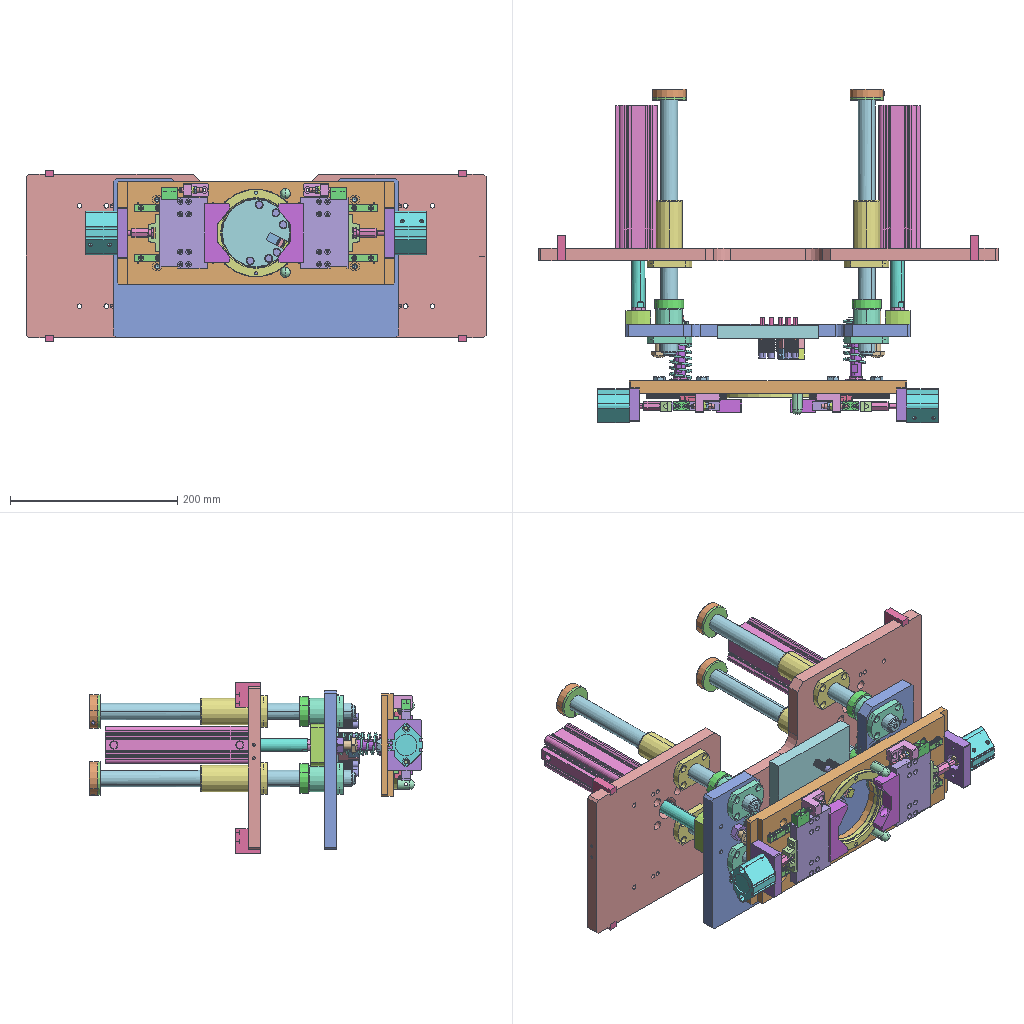Assembly | STEP file | 55 different items | 119 placed | box 550 x 399 x 205 mm
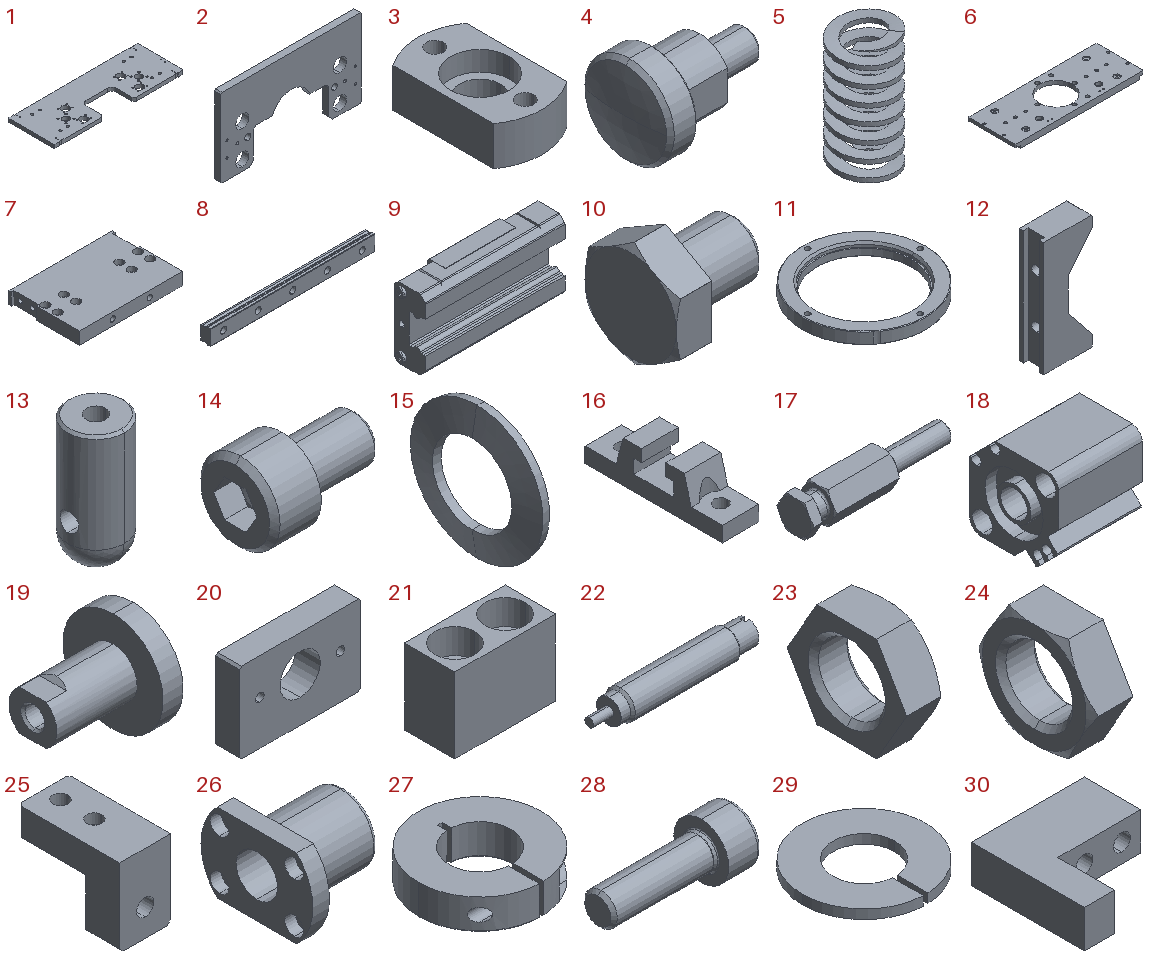Parts list (item | name | quantity | parent item | size | volume):
1 | PNXX056239 Base | x1 | in 23 | 550 x 195 x 15 mm | 1337407 mm3
2 | PNXX056238 Middle Base_Default | x1 | in 23 | 340 x 15 x 190 mm | 662186 mm3
3 | qnSceondFJMC8part4 | x2 | in qnSceondFJMC8-00_FJMC8 | 30 x 51 x 16 mm | 15639 mm3
4 | qnSceondFJMC8part5 | x2 | in qnSceondFJMC8-00_FJMC8 | 32 x 23 x 23 mm | 5961 mm3
5 | SWY24.5-55_Default | x2 | in 23 | 26.648 x 26.648 x 55 mm | 5041 mm3
6 | PNXX056237 Under Base | x1 | in qnSceondMove 1_Default | 332 x 122 x 15 mm | 468693 mm3
7 | PNXX056248 JIG Block | x2 | in qnSceondMove 1_Default | 84 x 57 x 10 mm | 44690 mm3
8 | 2SRS9MUU+95L | x4 | in 8 | 95 x 5.5 x 9 mm | 3697 mm3
9 | qnSceond_SRS9MQZUU Slider | x4 | in 8 | 40.8 x 9.1 x 20 mm | 5179 mm3
10 | STEHN13 | x4 | in qnSceondMove 1_Default | 15 x 13 x 15 mm | 1216 mm3
11 | PNXX056250 JIG_Default | x1 | in qnSceondMove 1_Default | 105 x 105 x 10 mm | 33679 mm3
12 | PNXX056247 JIG_Default | x2 | in qnSceondMove 1_Default | 30 x 15 x 70 mm | 19012 mm3
13 | PNXX056251 Pin_Default | x2 | in qnSceondMove 1_Default | 12 x 12 x 27 mm | 2502 mm3
14 | CB5-8_Default | x1 | in CB5-8_CW5_Default | 13 x 8.5 x 8.5 mm | 398.056 mm3
15 | CW5_Default | x1 | in CB5-8_CW5_Default | 0.85 x 9 x 9 mm | 22.263 mm3
16 | hlre7_2_03 | x2 | in qnSceondMove 1_Default | 12 x 45 x 13.5 mm | 3705 mm3
17 | fjdl6_1_0_4_20_2_03 | x2 | in qnSceondMove 1_Default | 46 x 11.547 x 10 mm | 2689 mm3
18 | 1_9 | x2 | in CDQ2B25-5DZ_0_0_0_ | 37.5 x 40 x 40 mm | 38658 mm3
19 | 2_9 | x2 | in CDQ2B25-5DZ_0_0_0_ | 25 x 25 x 25 mm | 4428 mm3
20 | PNXX056249 Cylinder BKT_Default | x2 | in qnSceondMove 1_Default | 60 x 12 x 40 mm | 24374 mm3
21 | PNXX056259 Stop Block_Default | x2 | in qnSceondMove 1_Default | 20 x 10 x 15 mm | 2179 mm3
22 | 1_10 | x2 | in RB0604_0_ | 32.5 x 6 x 6 mm | 755.606 mm3
23 | 2_10 | x2 | in RB0604_0_ | 3 x 9.238 x 8 mm | 99.469 mm3
24 | 3_1 | x2 | in RB0604_0_ | 3 x 9.238 x 8 mm | 99.469 mm3
25 | PNXX056261 Stop Block_Default | x2 | in qnSceondMove 1_Default | 15 x 30 x 23 mm | 5038 mm3
26 | qnslhfc20_2_03 | x4 | in 23 | 42 x 54 x 38 mm | 27385 mm3
27 | qnSceond1_10 | x4 | in qnSceondpscdj20_13_2_031 | 40 x 39.986 x 10 mm | 8415 mm3
28 | qnSceond2_10 | x4 | in qnSceondpscdj20_13_2_031 | 21 x 8.5 x 8.5 mm | 547.959 mm3
29 | qnSceond3_2 | x4 | in qnSceondpscdj20_13_2_031 | 40 x 39.986 x 3 mm | 2782 mm3
30 | PNXX056244 Stopper_Default | x4 | in 23 | 30 x 30 x 10 mm | 4879 mm3
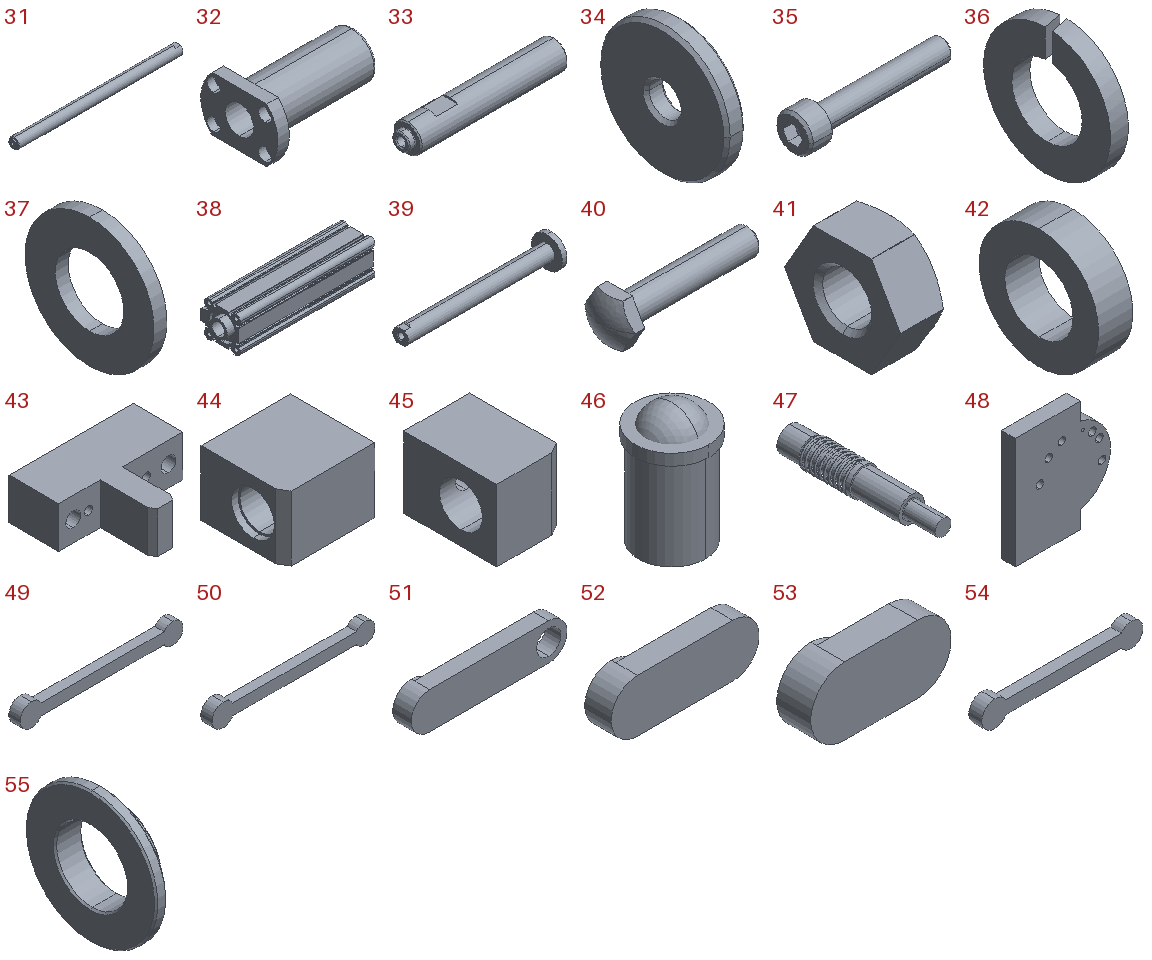31 | sfpg20_315_f3_p15_m6_sc305_2_03 | x4 | in 23 | 318 x 20 x 20 mm | 98846 mm3
32 | lhfcwmf20_2_03 | x4 | in 23 | 80 x 54 x 38 mm | 46009 mm3
33 | sfppa13_68_f3_p8_m5_n5_sc10_2_03 | x2 | in 23 | 71 x 13 x 13 mm | 8114 mm3
34 | wssb20_5_3_2_03 | x2 | in 23 | 3 x 20 x 20 mm | 863.938 mm3
35 | CB5-30_Default | x1 | in CB5-30_SW5_W5_Default | 35 x 8.5 x 8.5 mm | 830.025 mm3
36 | SW5_Default | x1 | in CB5-30_SW5_W5_Default | 1.3 x 9.2 x 9.198 mm | 58.481 mm3
37 | W5_Default | x1 | in CB5-30_SW5_W5_Default | 1 x 10 x 10 mm | 56.478 mm3
38 | 1 | x2 | in CDQ2A32-125DCZ | 175.5 x 49.5 x 45 mm | 171932 mm3
39 | 2 | x2 | in CDQ2A32-125DCZ | 157 x 32 x 32 mm | 34054 mm3
40 | 1_5 | x2 | in stbb10_50_2_03 | - | 5335 mm3
41 | 2_5 | x2 | in stbb10_50_2_03 | 8 x 19.6 x 17 mm | 1538 mm3
42 | urws35_20_10_2_03 | x4 | in 23 | 10 x 35 x 35 mm | 6480 mm3
43 | 22DDSceond144_Default | x1 | in 22DDSceondchatou_Default | 30 x 25 x 10 mm | 3740 mm3
44 | 22DDSceond4trr_Default | x1 | in 22DDSceondchatou_Default | 13.8 x 13 x 10 mm | 1356 mm3
45 | 22DDSceondwrwet_Default | x1 | in 22DDSceondchatou_Default | 9.2 x 13 x 10 mm | 888.519 mm3
46 | 22DDSceondZAL02-M6_Default | x2 | in 22DDSceondchatou_Default | 6.6 x 6.6 x 10.6 mm | 325.856 mm3
47 | 22CPMM160_Default | x6 | in 22DDSceoWWnd Terminal Inspection Tip sss_Default | 9.1 x 48.5 x 9.1 mm | 1897 mm3
48 | jjjj_Default | x1 | in 22DDSceoWWnd Terminal Inspection Tip sss_Default | 102.5 x 15 x 120 mm | 138148 mm3
49 | 222_Default | x1 | in 22DDSceoWWnd Terminal Inspection Tip sss_Default | 86.9 x 6 x 12 mm | 3087 mm3
50 | 333_Default | x1 | in 22DDSceoWWnd Terminal Inspection Tip sss_Default | 88.1 x 6 x 12 mm | 3123 mm3
51 | 444_Default | x1 | in 22DDSceoWWnd Terminal Inspection Tip sss_Default | 51 x 6 x 12 mm | 2767 mm3
52 | TYYUTI_Default | x1 | in 22DDSceoWWnd Terminal Inspection Tip sss_Default | 33.7 x 6 x 12 mm | 1981 mm3
53 | JTJTRUYIU_Default | x1 | in 22DDSceoWWnd Terminal Inspection Tip sss_Default | 24.8 x 6 x 12 mm | 1447 mm3
54 | 111_Default | x1 | in 22DDSceoWWnd Terminal Inspection Tip sss_Default | 75 x 6 x 12 mm | 2730 mm3
55 | ftcm_d16_5_h24_v13_0_t2_0_l5_0_2_03 | x4 | in 23 | 5 x 24 x 24 mm | 869.825 mm3
Placements (level | parent | child | x y z in mm | rotation matrix by rows):
1 | 23 | PNXX056239 Base | -0.0 -0.0 -0.0 | 1 0 0 0 0 1 0 -1 0
1 | 23 | PNXX056238 Middle Base_Default | 0.0 -90.985 5.0 | -1 0 0 0 1 0 0 0 -1
1 | 23 | qnSceondFJMC8-00_FJMC8 | -155.0 -59.985 35.0 | 1 0 0 0 0 -1 0 1 -0
2 | qnSceondFJMC8-00_FJMC8 | qnSceondFJMC8part4 | -0.0 -0.0 -0.0 | 1 0 0 0 1 0 0 0 1
2 | qnSceondFJMC8-00_FJMC8 | qnSceondFJMC8part5 | -0.0 -0.0 8.0 | 0 0 1 0 1 0 -1 0 0
1 | 23 | qnSceondFJMC8-00_FJMC8 | 155.0 -59.985 35.0 | 1 0 0 0 0 -1 0 1 0
2 | qnSceondFJMC8-00_FJMC8 | qnSceondFJMC8part4 | -0.0 -0.0 -0.0 | 1 0 0 0 1 0 0 0 1
2 | qnSceondFJMC8-00_FJMC8 | qnSceondFJMC8part5 | -0.0 -0.0 8.0 | 0 0 1 0 1 0 -1 0 0
1 | 23 | SWY24.5-55_Default | -104.767 -157.652 35.635 | -0.3446 -0.9387 0 0 0 1 -0.9387 0.3446 0
1 | 23 | qnSceondMove 1_Default | -0.0 -158.985 35.0 | 1 0 0 0 1 0 0 0 1
2 | qnSceondMove 1_Default | PNXX056237 Under Base | -0.0 -0.0 -0.0 | 1 0 0 0 0 1 0 -1 0
2 | qnSceondMove 1_Default | PNXX056248 JIG Block | -70.5 -10.0 0.0 | 0 -1 0 0 0 -1 1 0 -0
2 | qnSceondMove 1_Default | 2SRS9MUU+95L | -137.5 -0.0 -30.0 | 1 0 0 0 -1 0 0 0 -1
3 | 2SRS9MUU+95L | 2SRS9MUU+95L | -0.0 -0.0 -0.0 | 1 0 0 0 1 0 0 0 1
3 | 2SRS9MUU+95L | qnSceond_SRS9MQZUU Slider | 52.0 0.9 -0.0 | 1 0 0 0 1 0 0 0 1
2 | qnSceondMove 1_Default | 2SRS9MUU+95L | -137.5 -0.0 30.0 | 1 0 0 0 -1 0 0 0 -1
3 | 2SRS9MUU+95L | 2SRS9MUU+95L | -0.0 -0.0 -0.0 | 1 0 0 0 1 0 0 0 1
3 | 2SRS9MUU+95L | qnSceond_SRS9MQZUU Slider | 52.0 0.9 0.0 | 1 0 0 0 1 0 0 0 1
2 | qnSceondMove 1_Default | 2SRS9MUU+95L | 57.5 -0.0 -30.0 | 1 0 0 0 -1 0 0 0 -1
3 | 2SRS9MUU+95L | 2SRS9MUU+95L | -0.0 -0.0 -0.0 | 1 0 0 0 1 0 0 0 1
3 | 2SRS9MUU+95L | qnSceond_SRS9MQZUU Slider | 23.0 0.9 0.0 | 1 0 0 0 1 0 0 0 1
2 | qnSceondMove 1_Default | 2SRS9MUU+95L | 57.5 -0.0 30.0 | 1 0 0 0 -1 0 0 0 -1
3 | 2SRS9MUU+95L | 2SRS9MUU+95L | -0.0 -0.0 -0.0 | 1 0 0 0 1 0 0 0 1
3 | 2SRS9MUU+95L | qnSceond_SRS9MQZUU Slider | 23.0 0.9 -0.0 | 1 0 0 0 1 0 0 0 1
2 | qnSceondMove 1_Default | PNXX056248 JIG Block | 65.5 -10.0 -0.0 | 0 1 0 0 0 -1 -1 0 -0
2 | qnSceondMove 1_Default | STEHN13 | 78.0 15.0 -0.0 | 0 1 0 -1 0 0 0 0 1
2 | qnSceondMove 1_Default | STEHN13 | -78.0 15.0 0.0 | 0 0.1705 -0.9854 -1 0 0 0 0.9854 0.1705
2 | qnSceondMove 1_Default | PNXX056250 JIG_Default | -0.0 -5.0 0.0 | -1 0 0 0 0 -1 0 -1 0
2 | qnSceondMove 1_Default | PNXX056247 JIG_Default | -61.5 -22.5 0.0 | 1 0 0 0 1 0 0 0 1
2 | qnSceondMove 1_Default | PNXX056247 JIG_Default | 56.5 -22.5 -0.0 | -1 0 0 0 1 0 0 0 -1
2 | qnSceondMove 1_Default | PNXX056251 Pin_Default | 35.0 -25.0 47.0 | 1 0 0 0 0 1 0 -1 0
2 | qnSceondMove 1_Default | PNXX056251 Pin_Default | 35.0 -25.0 -47.0 | 1 0 0 0 0 1 0 -1 0
2 | qnSceondMove 1_Default | CB5-8_CW5_Default | -55.157 -13.625 14.645 | -1 0 0 0 -0.8471 -0.5315 0 -0.5315 0.8471
3 | CB5-8_CW5_Default | CB5-8_Default | -3.507 0.9755 1.032 | 1 0 0 0 1 0 0 0 1
3 | CB5-8_CW5_Default | CW5_Default | -3.507 0.9755 1.032 | 1 0 0 0 1 0 0 0 1
2 | qnSceondMove 1_Default | hlre7_2_03 | -115.5 -15.0 0.0 | 0 0 -1 -1 0 0 0 1 0
2 | qnSceondMove 1_Default | fjdl6_1_0_4_20_2_03 | -122.0 -15.0 0.0 | -1 0 0 0 0.9893 -0.1461 0 -0.1461 -0.9893
2 | qnSceondMove 1_Default | CDQ2B25-5DZ_0_0_0_ | -166.0 -15.0 0.0 | -1 0 0 0 -0.7071 -0.7071 0 -0.7071 0.7071
3 | CDQ2B25-5DZ_0_0_0_ | 1_9 | -0.0 -0.0 -0.0 | 1 0 0 0 1 0 0 0 1
3 | CDQ2B25-5DZ_0_0_0_ | 2_9 | -0.0 -0.0 -0.0 | 1 0 0 0 0.5826 0.8128 0 -0.8128 0.5826
2 | qnSceondMove 1_Default | PNXX056249 Cylinder BKT_Default | -154.0 -13.0 -0.0 | 0 -1 0 0 0 -1 1 0 -0
2 | qnSceondMove 1_Default | hlre7_2_03 | 110.5 -15.0 0.0 | 0 0 1 1 0 0 0 1 0
2 | qnSceondMove 1_Default | PNXX056249 Cylinder BKT_Default | 166.0 -13.0 -0.0 | 0 -1 0 0 0 -1 1 0 -0
2 | qnSceondMove 1_Default | CDQ2B25-5DZ_0_0_0_ | 166.0 -15.0 0.0 | 1 0 0 0 -0.7071 -0.7071 0 0.7071 -0.7071
3 | CDQ2B25-5DZ_0_0_0_ | 1_9 | -0.0 -0.0 -0.0 | 1 0 0 0 1 0 0 0 1
3 | CDQ2B25-5DZ_0_0_0_ | 2_9 | -5.0 -0.0 0.0 | 1 0 0 0 0.5857 -0.8105 0 0.8105 0.5857
2 | qnSceondMove 1_Default | fjdl6_1_0_4_20_2_03 | 117.0 -15.0 0.0 | 1 0 0 0 0.7867 -0.6173 0 0.6173 0.7867
2 | qnSceondMove 1_Default | PNXX056259 Stop Block_Default | -103.5 -20.0 47.5 | 1 0 0 0 1 0 0 0 1
2 | qnSceondMove 1_Default | PNXX056259 Stop Block_Default | 98.5 -20.0 47.5 | 1 0 0 0 1 0 0 0 1
2 | qnSceondMove 1_Default | RB0604_0_ | -92.0 -15.0 51.5 | 1 0 0 0 1 0 0 0 1
3 | RB0604_0_ | 1_10 | -0.0 -0.0 -0.0 | 1 0 0 0 1 0 0 0 1
3 | RB0604_0_ | 2_10 | -0.0 -0.0 -0.0 | 1 0 0 0 1 0 0 0 1
3 | RB0604_0_ | 3_1 | -0.0 -0.0 -0.0 | 1 0 0 0 1 0 0 0 1
2 | qnSceondMove 1_Default | PNXX056261 Stop Block_Default | -77.0 -8.0 44.0 | 0 1 0 0 0 1 1 0 0
2 | qnSceondMove 1_Default | PNXX056261 Stop Block_Default | 77.0 -8.0 59.0 | 0 -1 0 0 0 1 -1 0 0
2 | qnSceondMove 1_Default | RB0604_0_ | 92.0 -15.0 51.5 | -1 0 0 0 -0.09795 0.9952 0 0.9952 0.09795
3 | RB0604_0_ | 1_10 | -0.0 -0.0 -0.0 | 1 0 0 0 1 0 0 0 1
3 | RB0604_0_ | 2_10 | -0.0 -0.0 -0.0 | 1 0 0 0 1 0 0 0 1
3 | RB0604_0_ | 3_1 | -0.0 -0.0 -0.0 | 1 0 0 0 1 0 0 0 1
2 | qnSceondMove 1_Default | STEHN13 | -130.0 15.0 0.0 | 0 0.1705 -0.9854 -1 0 0 0 0.9854 0.1705
2 | qnSceondMove 1_Default | STEHN13 | 130.0 15.0 -0.0 | 0 0.1705 -0.9854 -1 0 0 0 0.9854 0.1705
1 | 23 | qnslhfc20_2_03 | -118.0 -98.985 75.0 | 0 1 0 1 0 0 0 0 -1
1 | 23 | qnslhfc20_2_03 | -118.0 -98.985 -5.0 | 0 1 0 1 0 0 0 0 -1
1 | 23 | qnslhfc20_2_03 | 118.0 -98.985 -5.0 | 0 1 0 1 0 0 0 0 -1
1 | 23 | qnslhfc20_2_03 | 118.0 -98.985 75.0 | 0 1 0 1 0 0 0 0 -1
1 | 23 | qnSceondpscdj20_13_2_031 | -118.0 200.031 -5.0 | 0.7871 -0.6168 0 0 0 -1 0.6168 0.7871 0
2 | qnSceondpscdj20_13_2_031 | qnSceond1_10 | -0.0 -0.0 -0.0 | 1 0 0 0 1 0 0 0 1
2 | qnSceondpscdj20_13_2_031 | qnSceond2_10 | -0.0 -0.0 -0.0 | 1 0 0 0 1 0 0 0 1
2 | qnSceondpscdj20_13_2_031 | qnSceond3_2 | -0.0 -0.0 -0.0 | 1 0 0 0 1 0 0 0 1
1 | 23 | qnSceondpscdj20_13_2_031 | -118.0 200.031 75.0 | 0.9991 0.04303 0 0 0 -1 -0.04303 0.9991 0
2 | qnSceondpscdj20_13_2_031 | qnSceond1_10 | -0.0 -0.0 -0.0 | 1 0 0 0 1 0 0 0 1
2 | qnSceondpscdj20_13_2_031 | qnSceond2_10 | -0.0 -0.0 -0.0 | 1 0 0 0 1 0 0 0 1
2 | qnSceondpscdj20_13_2_031 | qnSceond3_2 | -0.0 -0.0 -0.0 | 1 0 0 0 1 0 0 0 1
1 | 23 | qnSceondpscdj20_13_2_031 | 118.0 200.031 75.0 | 0.9975 -0.07033 0 0 0 -1 0.07033 0.9975 0
2 | qnSceondpscdj20_13_2_031 | qnSceond1_10 | -0.0 -0.0 -0.0 | 1 0 0 0 1 0 0 0 1
2 | qnSceondpscdj20_13_2_031 | qnSceond2_10 | -0.0 -0.0 -0.0 | 1 0 0 0 1 0 0 0 1
2 | qnSceondpscdj20_13_2_031 | qnSceond3_2 | -0.0 -0.0 -0.0 | 1 0 0 0 1 0 0 0 1
1 | 23 | qnSceondpscdj20_13_2_031 | 118.0 200.031 -5.0 | 0.6155 -0.7881 0 0 0 -1 0.7881 0.6155 0
2 | qnSceondpscdj20_13_2_031 | qnSceond1_10 | -0.0 -0.0 -0.0 | 1 0 0 0 1 0 0 0 1
2 | qnSceondpscdj20_13_2_031 | qnSceond2_10 | -0.0 -0.0 -0.0 | 1 0 0 0 1 0 0 0 1
2 | qnSceondpscdj20_13_2_031 | qnSceond3_2 | -0.0 -0.0 -0.0 | 1 0 0 0 1 0 0 0 1
1 | 23 | PNXX056244 Stopper_Default | -247.0 15.0 95.0 | 0 0 1 0 1 0 -1 0 0
1 | 23 | PNXX056244 Stopper_Default | -247.0 15.0 -80.0 | 0 0 -1 0 1 0 1 0 -0
1 | 23 | PNXX056244 Stopper_Default | 247.0 15.0 -80.0 | 0 0 -1 0 1 0 1 0 -0
1 | 23 | PNXX056244 Stopper_Default | 247.0 15.0 95.0 | 0 0 1 0 1 0 -1 0 0
1 | 23 | sfpg20_315_f3_p15_m6_sc305_2_03 | -118.0 -109.969 75.0 | 0 -0.007247 1 1 0 0 0 1 0.007247
1 | 23 | sfpg20_315_f3_p15_m6_sc305_2_03 | 118.0 -109.969 75.0 | 0 -0.7788 0.6273 1 0 0 0 0.6273 0.7788
1 | 23 | sfpg20_315_f3_p15_m6_sc305_2_03 | 118.0 -109.969 -5.0 | 0 -0.9856 0.1689 1 0 0 0 0.1689 0.9856
1 | 23 | sfpg20_315_f3_p15_m6_sc305_2_03 | -118.0 -109.969 -5.0 | 0 -0.7308 0.6826 1 0 0 0 0.6826 0.7308
1 | 23 | lhfcwmf20_2_03 | -118.0 -8.0 75.0 | 0 -1 0 1 0 0 0 0 1
1 | 23 | lhfcwmf20_2_03 | -118.0 -8.0 -5.0 | 0 -1 0 1 0 0 0 0 1
1 | 23 | lhfcwmf20_2_03 | 118.0 -8.0 -5.0 | 0 -1 0 1 0 0 0 0 1
1 | 23 | lhfcwmf20_2_03 | 118.0 -8.0 75.0 | 0 -1 0 1 0 0 0 0 1
1 | 23 | sfppa13_68_f3_p8_m5_n5_sc10_2_03 | -105.0 -143.985 35.0 | 0 -0.9725 -0.2329 1 0 0 0 -0.2329 0.9725
1 | 23 | sfppa13_68_f3_p8_m5_n5_sc10_2_03 | 105.0 -143.985 35.0 | 0 -0.9725 -0.2329 1 0 0 0 -0.2329 0.9725
1 | 23 | SWY24.5-55_Default | 104.42 -138.172 35.347 | 0.8577 -0.5141 0 0 0 1 -0.5141 -0.8577 0
1 | 23 | wssb20_5_3_2_03 | -105.0 -75.985 35.0 | 0 -1 0 1 0 0 0 0 1
1 | 23 | wssb20_5_3_2_03 | 105.0 -75.985 35.0 | 0 -1 0 1 0 0 0 0 1
1 | 23 | CB5-30_SW5_W5_Default | -105.0 -70.685 35.0 | 0 1 0 -1 0 0 0 0 1
2 | CB5-30_SW5_W5_Default | CB5-30_Default | -0.0 -0.0 -0.0 | 1 0 0 0 1 0 0 0 1
2 | CB5-30_SW5_W5_Default | SW5_Default | 0.65 -0.0 -0.0 | 1 0 0 0 1 0 0 0 1
2 | CB5-30_SW5_W5_Default | W5_Default | 1.8 -0.0 0.0 | 1 0 0 0 1 0 0 0 1
1 | 23 | CDQ2A32-125DCZ | -155.0 15.0 35.0 | 0 -1 0 1 0 0 0 0 1
2 | CDQ2A32-125DCZ | 1 | -0.0 -0.0 -0.0 | 1 0 0 0 1 0 0 0 1
2 | CDQ2A32-125DCZ | 2 | -53.985 0.0 0.0 | 1 0 0 0 0.9409 -0.3386 0 0.3386 0.9409
1 | 23 | CDQ2A32-125DCZ | 155.0 15.0 35.0 | 0 1 0 1 0 0 0 0 -1
2 | CDQ2A32-125DCZ | 1 | -0.0 -0.0 -0.0 | 1 0 0 0 1 0 0 0 1
2 | CDQ2A32-125DCZ | 2 | -53.985 -0.0 0.0 | 1 0 0 0 0.7786 -0.6275 0 0.6275 0.7786
1 | 23 | stbb10_50_2_03 | 130.0 -108.985 35.0 | 0 -1 0 1 0 0 0 0 1
2 | stbb10_50_2_03 | 1_5 | -0.0 -0.0 -0.0 | 1 0 0 0 1 0 0 0 1
2 | stbb10_50_2_03 | 2_5 | -11.0 -0.0 0.0 | 1 0 0 0 1 0 0 0 1
1 | 23 | stbb10_50_2_03 | -130.0 -108.985 35.0 | 0 -1 0 1 0 0 0 0 1
2 | stbb10_50_2_03 | 1_5 | -0.0 -0.0 -0.0 | 1 0 0 0 1 0 0 0 1
2 | stbb10_50_2_03 | 2_5 | -11.0 -0.0 0.0 | 1 0 0 0 1 0 0 0 1
1 | 23 | urws35_20_10_2_03 | 118.0 -56.985 -5.0 | 0 0.427 0.9043 1 0 0 0 0.9043 -0.427
1 | 23 | urws35_20_10_2_03 | 118.0 -56.985 75.0 | 0 0.427 0.9043 1 0 0 0 0.9043 -0.427
1 | 23 | urws35_20_10_2_03 | -118.0 -56.985 -5.0 | 0 0.427 0.9043 1 0 0 0 0.9043 -0.427
1 | 23 | urws35_20_10_2_03 | -118.0 -56.985 75.0 | 0 0.427 0.9043 1 0 0 0 0.9043 -0.427
1 | 23 | 22DDSceoWWnd Terminal Inspection Tip sss_Default | -0.0 -78.037 35.0 | 0 0 1 0 1 0 -1 0 -0
2 | 22DDSceoWWnd Terminal Inspection Tip sss_Default | 22DDSceondchatou_Default | -11.711 -61.586 75.411 | -0.4602 0 0.8878 0 1 0 -0.8878 0 -0.4602
3 | 22DDSceondchatou_Default | 22DDSceond144_Default | 29.685 46.586 41.842 | 1 0 0 0 1 0 0 0 1
3 | 22DDSceondchatou_Default | 22DDSceond4trr_Default | 40.085 28.086 36.842 | 1 0 0 0 1 0 0 0 1
3 | 22DDSceondchatou_Default | 22DDSceondwrwet_Default | 21.585 28.086 36.842 | 1 0 0 0 1 0 0 0 1
3 | 22DDSceondchatou_Default | 22DDSceondZAL02-M6_Default | 26.185 26.586 41.842 | 0 0 1 0.287 0.9579 0 -0.9579 0.287 0
3 | 22DDSceondchatou_Default | 22DDSceondZAL02-M6_Default | 33.185 26.586 41.842 | 0 0 -1 0.8197 0.5727 0 0.5727 -0.8197 -0
2 | 22DDSceoWWnd Terminal Inspection Tip sss_Default | 22CPMM160_Default | -33.753 13.0 3.833 | -0.9411 0 -0.3382 0 -1 0 -0.3382 0 0.9411
2 | 22DDSceoWWnd Terminal Inspection Tip sss_Default | 22CPMM160_Default | -24.208 13.0 23.808 | -0.01742 0 -0.9998 0 -1 0 -0.9998 0 0.01742
2 | 22DDSceoWWnd Terminal Inspection Tip sss_Default | 22CPMM160_Default | -9.892 13.0 32.483 | 0.2832 0 0.959 0 -1 0 0.959 0 -0.2832
2 | 22DDSceoWWnd Terminal Inspection Tip sss_Default | 22CPMM160_Default | 23.013 13.0 25.012 | 0.2832 0 0.959 0 -1 0 0.959 0 -0.2832
2 | 22DDSceoWWnd Terminal Inspection Tip sss_Default | 22CPMM160_Default | 30.464 13.0 15.11 | 0.4722 0 0.8815 0 -1 0 0.8815 0 -0.4722
2 | 22DDSceoWWnd Terminal Inspection Tip sss_Default | 22CPMM160_Default | 33.338 13.0 -6.841 | 0.2832 0 0.959 0 -1 0 0.959 0 -0.2832
2 | 22DDSceoWWnd Terminal Inspection Tip sss_Default | jjjj_Default | -0.0 -0.0 -0.0 | 1 0 0 0 1 0 0 0 1
2 | 22DDSceoWWnd Terminal Inspection Tip sss_Default | 222_Default | 0.217 -5.0 -7.456 | 0.8015 0 -0.598 0 1 0 0.598 0 0.8015
2 | 22DDSceoWWnd Terminal Inspection Tip sss_Default | 333_Default | 1.651 -5.0 -28.433 | 0.8264 0 -0.5631 0 1 0 0.5631 0 0.8264
2 | 22DDSceoWWnd Terminal Inspection Tip sss_Default | 444_Default | -27.341 -5.0 41.189 | 0.8948 0 0.4465 0 1 0 -0.4465 0 0.8948
2 | 22DDSceoWWnd Terminal Inspection Tip sss_Default | TYYUTI_Default | -34.607 -5.0 26.905 | 0.9584 0 0.2854 0 1 0 -0.2854 0 0.9584
2 | 22DDSceoWWnd Terminal Inspection Tip sss_Default | JTJTRUYIU_Default | -39.365 -5.0 6.91 | 0.8768 0 0.4808 0 1 0 -0.4808 0 0.8768
2 | 22DDSceoWWnd Terminal Inspection Tip sss_Default | 111_Default | -3.48 -5.0 7.514 | 0.8344 0 -0.5511 0 1 0 0.5511 0 0.8344
1 | 23 | ftcm_d16_5_h24_v13_0_t2_0_l5_0_2_03 | -105.0 -143.985 35.0 | 0 -1 0 1 0 0 0 0 1
1 | 23 | ftcm_d16_5_h24_v13_0_t2_0_l5_0_2_03 | 105.0 -143.985 35.0 | 0 -1 0 1 0 0 0 0 1
1 | 23 | ftcm_d16_5_h24_v13_0_t2_0_l5_0_2_03 | -105.0 -90.985 35.0 | 0 -0.3363 -0.9418 -1 0 0 0 0.9418 -0.3363
1 | 23 | ftcm_d16_5_h24_v13_0_t2_0_l5_0_2_03 | 105.0 -90.985 35.0 | 0 -0.4889 -0.8723 -1 0 0 0 0.8723 -0.4889